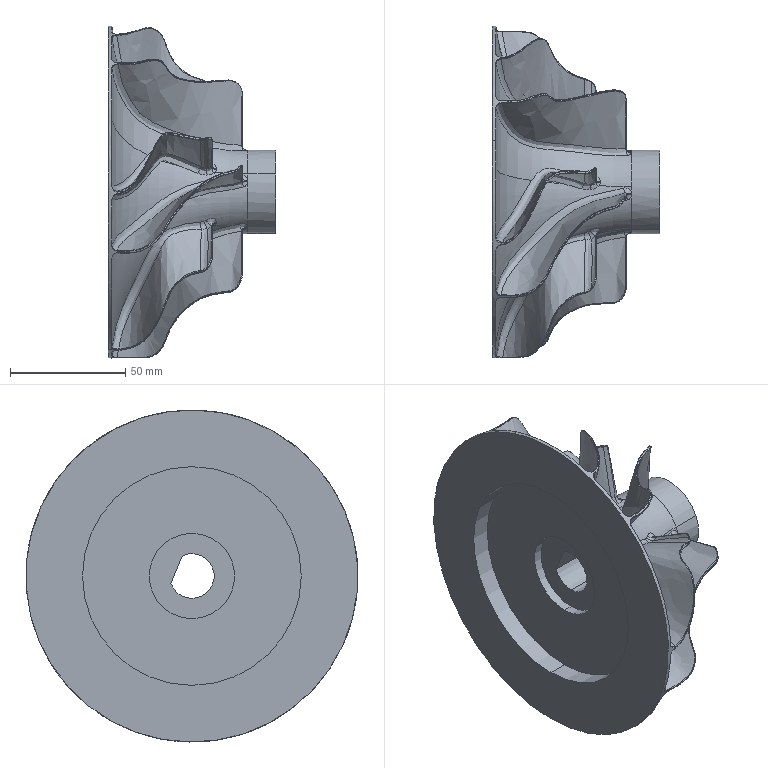Part | STEP file | Previa 01.sldasm-Part-1_Valor predeterminado | 1 solid | 366 faces | volume 182355 mm3 | spline 270 | torus 64 | cylinder 17 | plane 15 | commonest cylinder face diameters 98.252 x5 19.36 x3 144.232 x3 36.3 x2 37.038 x2 95.038 x2